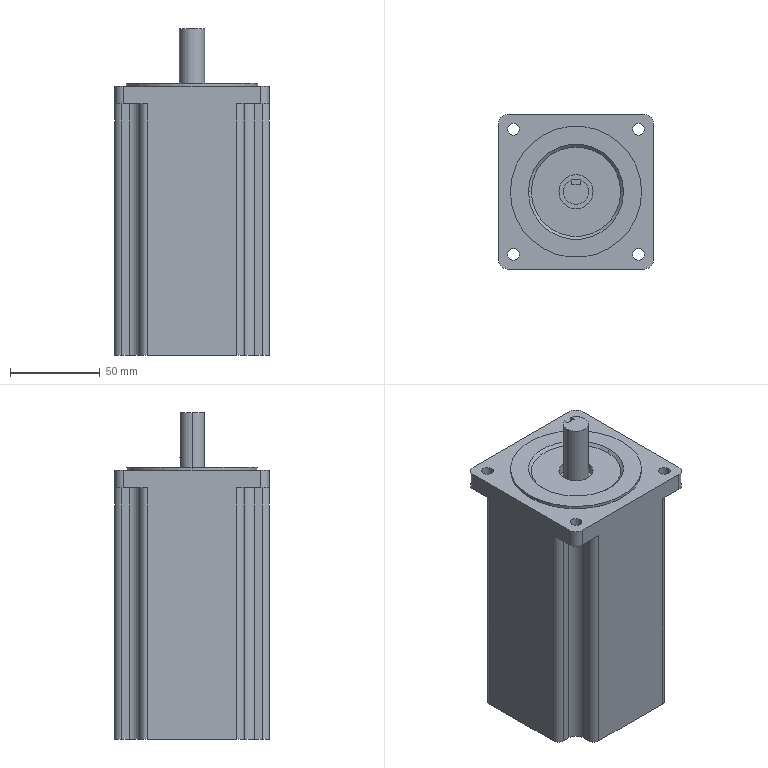Part | STEP file | LC86HS150(shaft 14 length 32)- | 1 solid | 58 faces | box 86 x 86 x 182 mm | volume 1005876 mm3 | cylinder 30 | plane 26 | cone 2 | commonest cylinder face diameters 6.5 x8 8 x8 10 x4 12 x4 14 x2 19 x2